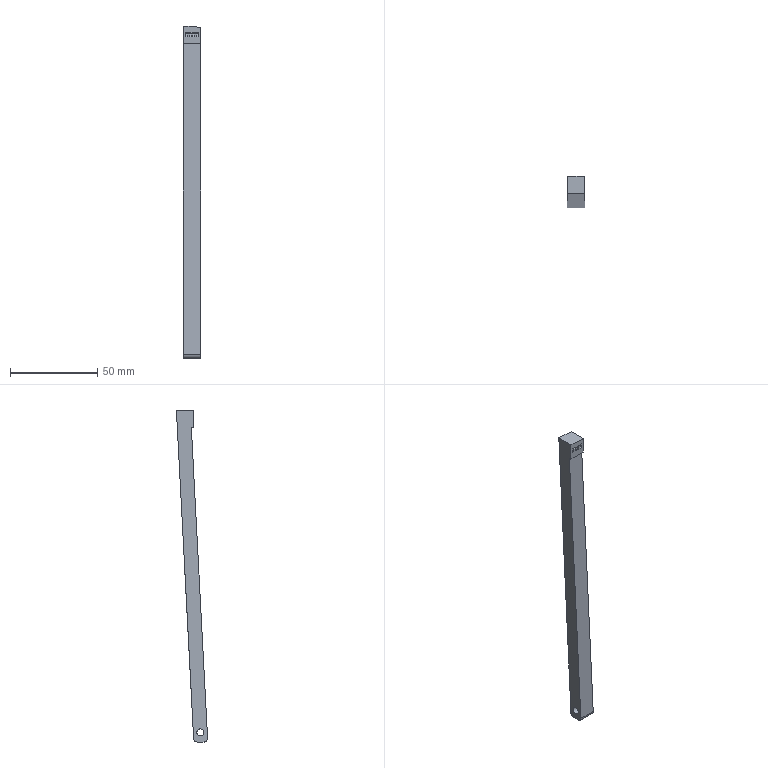Part | STEP file | solid 28 | 1 solid | 42 faces | box 10 x 17.865 x 190.084 mm | volume 15194 mm3 | plane 33 | cylinder 5 | other 4 | commonest cylinder face diameters 4 x3 1.005 x1 6922 x1